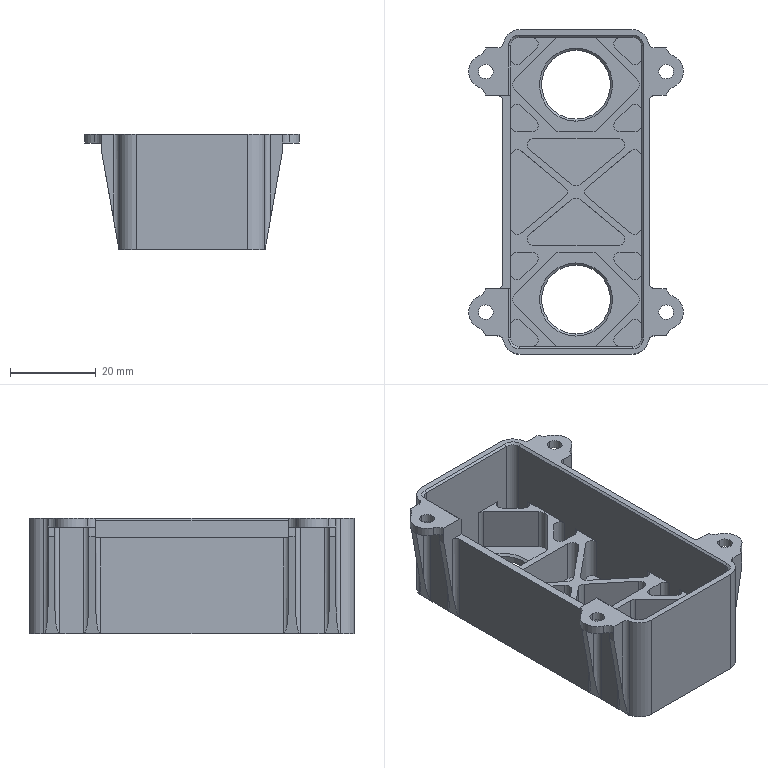NC program | NX | posted with a generic post | part box 50 x 75.58 x 26.8 mm
Lines 6158 to 6975 of 37241:
(ZLEVEL_PROFILE_COPY_1 , TOOL : D6)
N12284 T12 M6
N12286 G54
N12288 G17 G0 G90 X-31.649 Y21.375 S9500 M3
N12290 G43 Z30. H12
N12292 Z-0.992
N12294 G94 G1 X-31.331 Y20.514 F1000.
N12296 G3 X-30.87 Y20.131 R0.6
N12298 G2 X-30.375 Y20. R2.877 F1500.
N12300 G1 X-29.859
N12302 G3 X-29.34 Y20.3 R0.6
N12304 G1 X-28.82 Y21.2
N12306 G0 X-31.525 Y21.463 Z-1.488
N12308 G1 X-31.265 Y20.595 F1000.
N12310 G3 X-30.829 Y20.184 R0.6
N12312 G2 X-30.292 Y20. R2.948 F1500.
N12314 G1 X-29.702
N12316 G3 X-29.183 Y20.3 R0.6
N12318 G1 X-28.663 Y21.2
N12320 G0 X-31.389 Y21.544 Z-1.984
N12322 G1 X-31.177 Y20.662 F1000.
N12324 G3 X-30.764 Y20.227 R0.6
N12326 G2 X-30.208 Y20. R2.99 F1500.
N12328 G1 X-29.571
N12330 G3 X-29.051 Y20.3 R0.6
N12332 G1 X-28.531 Y21.2
N12334 G0 X-31.281 Y21.617 Z-2.48
N12336 G1 X-31.109 Y20.727 F1000.
N12338 G3 X-30.716 Y20.273 R0.6
N12340 G2 X-30.137 Y20. R2.98 F1500.
N12342 G1 X-29.444
N12344 G3 X-28.925 Y20.3 R0.6
N12346 G1 X-28.405 Y21.2
N12348 G0 X-31.183 Y21.686 Z-2.976
N12350 G1 X-31.049 Y20.79 F1000.
N12352 G3 X-30.675 Y20.321 R0.6
N12354 G2 X-30.075 Y20. R2.942 F1500.
N12356 G1 X-29.328
N12358 G3 X-28.809 Y20.3 R0.6
N12360 G1 X-28.289 Y21.2
N12362 G0 X-31.078 Y21.747 Z-3.472
N12364 G1 X-30.977 Y20.846 F1000.
N12366 G3 X-30.622 Y20.363 R0.6
N12368 G2 X-30.007 Y20. R2.977 F1500.
N12370 G1 X-29.216
N12372 G3 X-28.696 Y20.3 R0.6
N12374 G1 X-28.176 Y21.2
N12376 G0 X-30.98 Y21.806 Z-3.968
N12378 G1 X-30.912 Y20.902 F1000.
N12380 G3 X-30.574 Y20.406 R0.6
N12382 G2 X-29.946 Y20. R2.97 F1500.
N12384 G1 X-29.11
N12386 G3 X-28.59 Y20.3 R0.6
N12388 G1 X-28.07 Y21.2
N12390 G0 Z30.
N12392 X-27.167
N12394 Z-0.992
N12396 G1 X-26.647 Y20.3 F1000.
N12398 G3 X-26.128 Y20. R0.6
N12400 G1 X-25.625 F1500.
N12402 G2 X-25.14 Y20.129 R3.02
N12404 G3 X-24.681 Y20.515 R0.6
N12406 G1 X-24.37 Y21.375
N12408 G0 X-27.338 Y21.2 Z-1.488
N12410 G1 X-26.818 Y20.3 F1000.
N12412 G3 X-26.299 Y20. R0.6
N12414 G1 X-25.709 F1500.
N12416 G2 X-25.17 Y20.184 R2.919
N12418 G3 X-24.734 Y20.596 R0.6
N12420 G1 X-24.474 Y21.462
N12422 G0 X-27.469 Y21.2 Z-1.984
N12424 G1 X-26.949 Y20.3 F1000.
N12426 G3 X-26.43 Y20. R0.6
N12428 G1 X-25.788 F1500.
N12430 G2 X-25.23 Y20.229 R2.964
N12432 G3 X-24.816 Y20.664 R0.6
N12434 G1 X-24.604 Y21.544
N12436 G0 X-27.595 Y21.2 Z-2.48
N12438 G1 X-27.075 Y20.3 F1000.
N12440 G3 X-26.556 Y20. R0.6
N12442 G1 X-25.86 F1500.
N12444 G2 X-25.279 Y20.275 R2.952
N12446 G3 X-24.886 Y20.728 R0.6
N12448 G1 X-24.715 Y21.618
N12450 G0 X-27.712 Y21.2 Z-2.976
N12452 G1 X-27.193 Y20.3 F1000.
N12454 G3 X-26.673 Y20. R0.6
N12456 G1 X-25.926 F1500.
N12458 G2 X-25.323 Y20.321 R2.959
N12460 G3 X-24.949 Y20.79 R0.6
N12462 G1 X-24.814 Y21.686
N12464 G0 X-27.823 Y21.2 Z-3.472
N12466 G1 X-27.304 Y20.3 F1000.
N12468 G3 X-26.784 Y20. R0.6
N12470 G1 X-25.994 F1500.
N12472 G2 X-25.38 Y20.362 R2.976
N12474 G3 X-25.024 Y20.845 R0.6
N12476 G1 X-24.924 Y21.746
N12478 G0 X-27.929 Y21.2 Z-3.968
N12480 G1 X-27.41 Y20.3 F1000.
N12482 G3 X-26.89 Y20. R0.6
N12484 G1 X-26.054 F1500.
N12486 G2 X-25.427 Y20.406 R2.97
N12488 G3 X-25.089 Y20.902 R0.6
N12490 G1 X-25.021 Y21.805
N12492 G0 X-28.034 Y21.2 Z-4.464
N12494 G1 X-27.514 Y20.3 F1000.
N12496 G3 X-26.995 Y20. R0.6
N12498 G1 X-26.115 F1500.
N12500 G2 X-25.474 Y20.45 R2.985
N12502 G3 X-25.152 Y20.956 R0.6
N12504 G1 X-25.112 Y21.862
N12506 G0 Z30.
N12508 X-30.888
N12510 Z-4.464
N12512 G1 X-30.848 Y20.956 F1000.
N12514 G3 X-30.526 Y20.45 R0.6
N12516 G2 X-29.885 Y20. R2.985 F1500.
N12518 G1 X-29.005
N12520 G3 X-28.486 Y20.3 R0.6
N12522 G1 X-27.966 Y21.2
N12524 G0 X-30.79 Y21.915 Z-4.96
N12526 G1 X-30.779 Y21.008 F1000.
N12528 G3 X-30.473 Y20.492 R0.6
N12530 G2 X-29.824 Y20. R2.991 F1500.
N12532 G1 X-28.904
N12534 G3 X-28.384 Y20.3 R0.6
N12536 G1 X-27.865 Y21.2
N12538 G0 Z30.
N12540 X-28.135
N12542 Z-4.96
N12544 G1 X-27.615 Y20.3 F1000.
N12546 G3 X-27.096 Y20. R0.6
N12548 G1 X-26.176 F1500.
N12550 G2 X-25.529 Y20.491 R2.984
N12552 G3 X-25.223 Y21.007 R0.6
N12554 G1 X-25.213 Y21.914
N12556 G0 X-28.235 Y21.2 Z-5.456
N12558 G1 X-27.716 Y20.3 F1000.
N12560 G3 X-27.196 Y20. R0.6
N12562 G1 X-26.236 F1500.
N12564 G2 X-25.587 Y20.533 R2.969
N12566 G3 X-25.298 Y21.058 R0.6
N12568 G1 X-25.317 Y21.964
N12570 G0 Z30.
N12572 X-30.691 Y21.965
N12574 Z-5.456
N12576 G1 X-30.708 Y21.058 F1000.
N12578 G3 X-30.417 Y20.533 R0.6
N12580 G2 X-29.764 Y20. R2.988 F1500.
N12582 G1 X-28.804
N12584 G3 X-28.285 Y20.3 R0.6
N12586 G1 X-27.765 Y21.2
N12588 G0 X-30.593 Y22.014 Z-5.952
N12590 G1 X-30.636 Y21.108 F1000.
N12592 G3 X-30.362 Y20.575 R0.6
N12594 G2 X-29.703 Y20. R2.988 F1500.
N12596 G1 X-28.705
N12598 G3 X-28.185 Y20.3 R0.6
N12600 G1 X-27.666 Y21.2
N12602 G0 Z30.
N12604 X-28.334
N12606 Z-5.952
N12608 G1 X-27.815 Y20.3 F1000.
N12610 G3 X-27.295 Y20. R0.6
N12612 G1 X-26.297 F1500.
N12614 G2 X-25.646 Y20.573 R2.962
N12616 G3 X-25.373 Y21.108 R0.6
N12618 G1 X-25.419 Y22.013
N12620 G0 X-28.433 Y21.2 Z-6.448
N12622 G1 X-27.913 Y20.3 F1000.
N12624 G3 X-27.394 Y20. R0.6
N12626 G1 X-26.358 F1500.
N12628 G2 X-25.7 Y20.615 R2.983
N12630 G3 X-25.441 Y21.156 R0.6
N12632 G1 X-25.51 Y22.061
N12634 G0 Z30.
N12636 X-30.497 Y22.062
N12638 Z-6.448
N12640 G1 X-30.564 Y21.157 F1000.
N12642 G3 X-30.304 Y20.617 R0.6
N12644 G2 X-29.642 Y20. R2.997 F1500.
N12646 G1 X-28.606
N12648 G3 X-28.086 Y20.3 R0.6
N12650 G1 X-27.567 Y21.2
N12652 G0 X-30.401 Y22.108 Z-6.944
N12654 G1 X-30.492 Y21.206 F1000.
N12656 G3 X-30.246 Y20.659 R0.6
N12658 G2 X-29.58 Y20. R3.004 F1500.
N12660 G1 X-28.507
N12662 G3 X-27.988 Y20.3 R0.6
N12664 G1 X-27.468 Y21.2
N12666 G0 Z30.
N12668 X-28.532
N12670 Z-6.944
N12672 G1 X-28.012 Y20.3 F1000.
N12674 G3 X-27.493 Y20. R0.6
N12676 G1 X-26.42 F1500.
N12678 G2 X-25.76 Y20.657 R2.99
N12680 G3 X-25.514 Y21.204 R0.6
N12682 G1 X-25.608 Y22.107
N12684 G0 X-28.629 Y21.2 Z-7.44
N12686 G1 X-28.109 Y20.3 F1000.
N12688 G3 X-27.59 Y20. R0.6
N12690 G1 X-26.479 F1500.
N12692 G2 X-25.817 Y20.699 R2.993
N12694 G3 X-25.586 Y21.253 R0.6
N12696 G1 X-25.701 Y22.153
N12698 G0 Z30.
N12700 X-30.307 Y22.155
N12702 Z-7.44
N12704 G1 X-30.42 Y21.255 F1000.
N12706 G3 X-30.188 Y20.702 R0.6
N12708 G2 X-29.521 Y20. R2.998 F1500.
N12710 G1 X-28.41
N12712 G3 X-27.89 Y20.3 R0.6
N12714 G1 X-27.371 Y21.2
N12716 G0 X-30.204 Y22.195 Z-7.936
N12718 G1 X-30.342 Y21.299 F1000.
N12720 G3 X-30.124 Y20.74 R0.6
N12722 G2 X-29.465 Y20. R2.996 F1500.
N12724 G1 X-28.319
N12726 G3 X-27.799 Y20.3 R0.6
N12728 G1 X-27.279 Y21.2
N12730 G0 Z30.
N12732 X-28.722
N12734 Z-7.936
N12736 G1 X-28.202 Y20.3 F1000.
N12738 G3 X-27.682 Y20. R0.6
N12740 G1 X-26.535 F1500.
N12742 G2 X-25.874 Y20.741 R2.994
N12744 G3 X-25.657 Y21.3 R0.6
N12746 G1 X-25.794 Y22.197
N12748 G0 X-28.839 Y21.251 Z-8.432
N12750 G1 X-28.29 Y20.3 F1000.
N12752 G3 X-27.771 Y20. R0.6
N12754 G1 X-26.588 F1500.
N12756 G2 X-25.932 Y20.781 R2.996
N12758 G3 X-25.728 Y21.345 R0.6
N12760 G1 X-25.888 Y22.238
N12762 G0 Z30.
N12764 X-30.115 Y22.24
N12766 Z-8.432
N12768 G1 X-30.274 Y21.347 F1000.
N12770 G3 X-30.07 Y20.782 R0.6
N12772 G2 X-29.412 Y20. R2.996 F1500.
N12774 G1 X-28.229
N12776 G3 X-27.709 Y20.3 R0.6
N12778 G1 X-27.159 Y21.253
N12780 G0 X-30.015 Y22.275 Z-8.928
N12782 G1 X-30.198 Y21.386 F1000.
N12784 G3 X-30.008 Y20.817 R0.6
N12786 G2 X-29.36 Y20. R3.005 F1500.
N12788 G1 X-28.145
N12790 G3 X-27.626 Y20.3 R0.6
N12792 G1 X-26.831 Y21.676
N12794 G0 Z30.
N12796 X-29.169
N12798 Z-8.928
N12800 G1 X-28.374 Y20.3 F1000.
N12802 G3 X-27.855 Y20. R0.6
N12804 G1 X-26.64 F1500.
N12806 G2 X-25.992 Y20.817 R3.005
N12808 G3 X-25.802 Y21.386 R0.6
N12810 G1 X-25.985 Y22.275
N12812 G0 X-29.426 Y21.98 Z-9.424
N12814 G1 X-28.456 Y20.3 F1000.
N12816 G3 X-27.936 Y20. R0.6
N12818 G1 X-26.684 F1500.
N12820 G2 X-26.04 Y20.861 R2.998
N12822 G3 X-25.863 Y21.434 R0.6
N12824 G1 X-26.065 Y22.319
N12826 G0 Z30.
N12828 X-29.935
N12830 Z-9.424
N12832 G1 X-30.137 Y21.434 F1000.
N12834 G3 X-29.96 Y20.861 R0.6
N12836 G2 X-29.316 Y20. R2.998 F1500.
N12838 G1 X-28.064
N12840 G3 X-27.544 Y20.3 R0.6
N12842 G1 X-26.574 Y21.98
N12844 G0 X-29.848 Y22.355 Z-9.92
N12846 G1 X-30.071 Y21.476 F1000.
N12848 G3 X-29.908 Y20.898 R0.6
N12850 G2 X-29.273 Y20. R3.004 F1500.
N12852 G1 X-26.727
N12854 G2 X-26.092 Y20.898 R3.004
N12856 G3 X-25.929 Y21.475 R0.6
N12858 G1 X-26.152 Y22.355
N12860 G0 X-29.772 Y22.396 Z-10.416
N12862 G1 X-30.014 Y21.521 F1000.
N12864 G3 X-29.863 Y20.941 R0.6
N12866 G2 X-29.236 Y20. R3. F1500.
N12868 G1 X-26.765
N12870 G2 X-26.13 Y20.948 R3.003
N12872 G3 X-25.977 Y21.528 R0.6
N12874 G1 X-26.216 Y22.403
N12876 G0 X-29.685 Y22.428 Z-10.912
N12878 G1 X-29.948 Y21.559 F1000.
N12880 G3 X-29.812 Y20.975 R0.6
N12882 G2 X-29.199 Y20. R3.004 F1500.
N12884 G1 X-26.801
N12886 G2 X-26.188 Y20.975 R3.004
N12888 G3 X-26.052 Y21.56 R0.6
N12890 G1 X-26.314 Y22.428
N12892 G0 X-29.634 Y22.481 Z-11.408
N12894 G1 X-29.91 Y21.617 F1000.
N12896 G3 X-29.782 Y21.031 R0.6
N12898 G2 X-29.168 Y20. R3. F1500.
N12900 G1 X-26.832
N12902 G2 X-26.218 Y21.031 R3.
N12904 G3 X-26.09 Y21.617 R0.6
N12906 G1 X-26.366 Y22.481
N12908 G0 X-29.635 Y22.569 Z-11.904
N12910 G1 X-29.91 Y21.704 F1000.
N12912 G3 X-29.782 Y21.118 R0.6
N12914 G2 X-29.139 Y20. R3.002 F1500.
N12916 G1 X-26.861
N12918 G2 X-26.218 Y21.118 R3.003
N12920 G3 X-26.09 Y21.704 R0.6
N12922 G1 X-26.366 Y22.568
N12924 G0 X-29.636 Y22.657 Z-12.4
N12926 G1 X-29.912 Y21.793 F1000.
N12928 G3 X-29.783 Y21.206 R0.6
N12930 G2 X-29.113 Y20. R3.002 F1500.
N12932 G1 X-26.887
N12934 G2 X-26.216 Y21.207 R3.002
N12936 G3 X-26.088 Y21.793 R0.6
N12938 G1 X-26.363 Y22.657
N12940 G0 X-29.635 Y22.744 Z-12.896
N12942 G1 X-29.91 Y21.88 F1000.
N12944 G3 X-29.783 Y21.293 R0.6
N12946 G2 X-29.09 Y20. R3. F1500.
N12948 G1 X-26.91
N12950 G2 X-26.217 Y21.294 R3.
N12952 G3 X-26.089 Y21.88 R0.6
N12954 G1 X-26.365 Y22.744
N12956 G0 X-29.634 Y22.831 Z-13.392
N12958 G1 X-29.91 Y21.967 F1000.
N12960 G3 X-29.782 Y21.38 R0.6
N12962 G2 X-29.069 Y20. R3.001 F1500.
N12964 G1 X-26.931
N12966 G2 X-26.218 Y21.381 R3.001
N12968 G3 X-26.09 Y21.967 R0.6
N12970 G1 X-26.366 Y22.831
N12972 G0 X-29.636 Y22.92 Z-13.888
N12974 G1 X-29.912 Y22.055 F1000.
N12976 G3 X-29.783 Y21.469 R0.6
N12978 G2 X-29.052 Y20. R3. F1500.
N12980 G1 X-26.949
N12982 G2 X-26.217 Y21.468 R3.002
N12984 G3 X-26.089 Y22.055 R0.6
N12986 G1 X-26.364 Y22.919
N12988 G0 X-29.636 Y23.007 Z-14.384
N12990 G1 X-29.912 Y22.142 F1000.
N12992 G3 X-29.783 Y21.556 R0.6
N12994 G2 X-29.036 Y20. R3.004 F1500.
N12996 G1 X-26.964
N12998 G2 X-26.216 Y21.556 R3.003
N13000 G3 X-26.088 Y22.142 R0.6
N13002 G1 X-26.363 Y23.007
N13004 G0 X-29.636 Y23.095 Z-14.88
N13006 G1 X-29.912 Y22.231 F1000.
N13008 G3 X-29.784 Y21.645 R0.6
N13010 G2 X-29.026 Y20. R2.996 F1500.
N13012 G1 X-26.974
N13014 G2 X-26.216 Y21.645 R2.996
N13016 G3 X-26.088 Y22.231 R0.6
N13018 G1 X-26.363 Y23.095
N13020 G0 X-29.638 Y23.184 Z-15.376
N13022 G1 X-29.914 Y22.32 F1000.
N13024 G3 X-29.786 Y21.734 R0.6
N13026 G2 X-29.019 Y20. R2.992 F1500.
N13028 G1 X-26.981
N13030 G2 X-26.214 Y21.734 R2.992
N13032 G3 X-26.086 Y22.32 R0.6
N13034 G1 X-26.362 Y23.184
N13036 G0 X-29.637 Y23.27 Z-15.872
N13038 G1 X-29.912 Y22.406 F1000.
N13040 G3 X-29.784 Y21.819 R0.6
N13042 G2 X-29.008 Y20. R3. F1500.
N13044 G1 X-26.992
N13046 G2 X-26.216 Y21.82 R3.
N13048 G3 X-26.087 Y22.406 R0.6
N13050 G1 X-26.362 Y23.27
N13052 G0 X-29.642 Y23.361 Z-16.368
N13054 G1 X-29.916 Y22.496 F1000.
N13056 G3 X-29.787 Y21.91 R0.6
N13058 G2 X-29.003 Y20. R3.001 F1500.
N13060 G1 X-26.997
N13062 G2 X-26.179 Y21.946 R3.001
N13064 G3 X-26.04 Y22.53 R0.6
N13066 G1 X-26.3 Y23.399
N13068 G0 X-29.635 Y23.444 Z-16.864
N13070 G1 X-29.911 Y22.579 F1000.
N13072 G3 X-29.783 Y21.993 R0.6
N13074 G2 X-29. Y20.033 R3.004 F1500.
N13076 G1 Y20.
N13078 X-27.
N13080 G2 X-26.217 Y21.993 R3.003
N13082 G3 X-26.089 Y22.579 R0.6
N13084 G1 X-26.364 Y23.444
N13086 G0 X-29.647 Y23.537 Z-17.36
N13088 G1 X-29.92 Y22.672 F1000.
N13090 G3 X-29.79 Y22.086 R0.6
N13092 G2 X-29. Y20.061 R3.006 F1500.
N13094 G1 Y20.
N13096 X-27.
N13098 Y20.061
N13100 G2 X-26.209 Y22.087 R3.007
N13102 G3 X-26.079 Y22.673 R0.6
N13104 G1 X-26.351 Y23.538
N13106 G0 X-29.637 Y23.62 Z-17.856
N13108 G1 X-29.912 Y22.755 F1000.
N13110 G3 X-29.784 Y22.169 R0.6
N13112 G2 X-29. Y20.149 R3.003 F1500.
N13114 G1 Y20.
N13116 X-27.
N13118 Y20.149
N13120 G2 X-26.214 Y22.171 R3.004
N13122 G3 X-26.085 Y22.757 R0.6
N13124 G1 X-26.359 Y23.622
N13126 G0 X-29.629 Y23.703 Z-18.352
N13128 G1 X-29.906 Y22.839 F1000.
N13130 G3 X-29.779 Y22.252 R0.6
N13132 G2 X-29. Y20.236 R3. F1500.
N13134 G1 Y20.
N13136 X-27.
N13138 Y20.236
N13140 G2 X-26.221 Y22.253 R3.
N13142 G3 X-26.094 Y22.839 R0.6
N13144 G1 X-26.371 Y23.703
N13146 G0 X-29.629 Y23.79 Z-18.848
N13148 G1 X-29.906 Y22.926 F1000.
N13150 G3 X-29.779 Y22.34 R0.6
N13152 G2 X-29. Y20.323 R3. F1500.
N13154 G1 Y20.
N13156 X-27.
N13158 Y20.323
N13160 G2 X-26.221 Y22.34 R3.
N13162 G3 X-26.094 Y22.926 R0.6
N13164 G1 X-26.371 Y23.79
N13166 G0 X-29.648 Y23.887 Z-19.344
N13168 G1 X-29.92 Y23.022 F1000.
N13170 G3 X-29.79 Y22.436 R0.6
N13172 G2 X-29. Y20.411 R3.006 F1500.
N13174 G1 Y20.
N13176 X-27.
N13178 Y20.411
N13180 G2 X-26.208 Y22.437 R3.007
N13182 G3 X-26.078 Y23.023 R0.6
N13184 G1 X-26.35 Y23.888
N13186 G0 X-29.637 Y23.969 Z-19.84
N13188 G1 X-29.912 Y23.105 F1000.
N13190 G3 X-29.784 Y22.519 R0.6
N13192 G2 X-29. Y20.498 R3.003 F1500.
N13194 G1 Y20.
N13196 X-27.
N13198 Y20.498
N13200 G2 X-26.214 Y22.52 R3.004
N13202 G3 X-26.086 Y23.106 R0.6
N13204 G1 X-26.36 Y23.971
N13206 G0 X-29.637 Y24.057 Z-20.336
N13208 G1 X-29.912 Y23.192 F1000.
N13210 G3 X-29.784 Y22.606 R0.6
N13212 G2 X-29.03 Y21. R3.002 F1500.
N13214 G1 X-29. Y20.586
N13216 Y20.
N13218 X-27.
N13220 Y20.586
N13222 G2 X-26.221 Y22.602 R3.
N13224 G3 X-26.094 Y23.189 R0.6
N13226 G1 X-26.371 Y24.053
N13228 G0 X-29.638 Y24.144 Z-20.832
N13230 G1 X-29.913 Y23.28 F1000.
N13232 G3 X-29.784 Y22.694 R0.6
N13234 G2 X-29. Y20.673 R3.003 F1500.
N13236 G1 Y20.
N13238 X-27.
N13240 Y20.673
N13242 G2 X-26.212 Y22.697 R3.005
N13244 G3 X-26.083 Y23.283 R0.6
N13246 G1 X-26.356 Y24.148
N13248 G0 X-29.653 Y24.24 Z-21.328
N13250 G1 X-29.925 Y23.374 F1000.
N13252 G3 X-29.794 Y22.789 R0.6
N13254 G2 X-29. Y20.761 R3.008 F1500.
N13256 G1 Y20.
N13258 X-27.
N13260 Y20.761
N13262 G2 X-26.208 Y22.787 R3.007
N13264 G3 X-26.078 Y23.373 R0.6
N13266 G1 X-26.35 Y24.238
N13268 G0 X-29.661 Y24.331 Z-21.824
N13270 G1 X-29.93 Y23.465 F1000.
N13272 G3 X-29.798 Y22.879 R0.6
N13274 G2 X-29. Y20.848 R3.011 F1500.
N13276 G1 Y20.
N13278 X-27.
N13280 Y20.848
N13282 G2 X-26.214 Y22.87 R3.004
N13284 G3 X-26.085 Y23.456 R0.6
N13286 G1 X-26.359 Y24.321
N13288 G0 X-29.637 Y24.407 Z-22.32
N13290 G1 X-29.912 Y23.542 F1000.
N13292 G3 X-29.784 Y22.956 R0.6
N13294 G2 X-29. Y20.881 R3.004 F1500.
N13296 G1 Y20.
N13298 X-27.
N13300 Y20.936
N13302 G2 X-26.221 Y22.952 R3.
N13304 G3 X-26.094 Y23.539 R0.6
N13306 G1 X-26.371 Y24.403
N13308 G0 X-29.629 Y24.467 Z-22.816
N13310 G1 X-29.906 Y23.603 F1000.
N13312 G3 X-29.779 Y23.017 R0.6
N13314 G2 X-29. Y21. R3. F1500.
N13316 G1 Y20.
N13318 X-27.
N13320 Y21.
N13322 G2 X-26.221 Y23.017 R3.
N13324 G3 X-26.094 Y23.603 R0.6
N13326 G1 X-26.371 Y24.467
N13328 G0 X-29.629 Z-23.312
N13330 G1 X-29.906 Y23.603 F1000.
N13332 G3 X-29.779 Y23.017 R0.6
N13334 G2 X-29. Y21. R3. F1500.
N13336 G1 Y20.
N13338 X-27.
N13340 Y21.
N13342 G2 X-26.221 Y23.017 R3.
N13344 G3 X-26.094 Y23.603 R0.6
N13346 G1 X-26.371 Y24.467
N13348 G0 X-29.629 Z-23.808
N13350 G1 X-29.906 Y23.603 F1000.
N13352 G3 X-29.779 Y23.017 R0.6
N13354 G2 X-29. Y21. R3. F1500.
N13356 G1 Y20.
N13358 X-27.
N13360 Y21.
N13362 G2 X-26.221 Y23.017 R3.
N13364 G3 X-26.094 Y23.603 R0.6
N13366 G1 X-26.371 Y24.467
N13368 G0 X-29.629 Z-24.304
N13370 G1 X-29.906 Y23.603 F1000.
N13372 G3 X-29.779 Y23.017 R0.6
N13374 G2 X-29. Y21. R3. F1500.
N13376 G1 Y20.
N13378 X-27.
N13380 Y21.
N13382 G2 X-26.221 Y23.017 R3.
N13384 G3 X-26.094 Y23.603 R0.6
N13386 G1 X-26.371 Y24.467
N13388 G0 X-29.629 Z-24.8
N13390 G1 X-29.906 Y23.603 F1000.
N13392 G3 X-29.779 Y23.017 R0.6
N13394 G2 X-29. Y21. R3. F1500.
N13396 G1 Y20.
N13398 X-27.
N13400 Y21.
N13402 G2 X-26.221 Y23.017 R3.
N13404 G3 X-26.094 Y23.603 R0.6
N13406 G1 X-26.371 Y24.467
N13408 G0 Z30.
N13410 X-37.396 Y20.364
N13412 Z-1.984
N13414 G1 X-36.665 Y19.73 F1000.
N13416 G3 X-36.076 Y19.616 R0.6
N13418 G2 X-35.573 Y19.769 R7. F1500.
N13420 G1 X-35.468 Y19.846
N13422 G2 X-35.131 Y20.041 R2.974
N13424 G3 X-34.799 Y20.541 R0.6
N13426 G1 X-34.741 Y21.445
N13428 G0 X-37.507 Y20.309 Z-2.48
N13430 G1 X-36.767 Y19.686 F1000.
N13432 G3 X-36.176 Y19.581 R0.6
N13434 G2 X-35.643 Y19.75 R7. F1500.
N13436 X-35.193 Y20.063 R2.921
N13438 G3 X-34.887 Y20.579 R0.6
N13440 G1 X-34.876 Y21.484
N13442 G0 X-37.606 Y20.258 Z-2.976
N13444 G1 X-36.857 Y19.645 F1000.
N13446 G3 X-36.265 Y19.548 R0.6
N13448 G2 X-35.703 Y19.734 R7. F1500.
N13450 X-35.242 Y20.083 R2.971
N13452 G3 X-34.957 Y20.611 R0.6
N13454 G1 X-34.983 Y21.517
N13456 G0 X-37.708 Y20.204 Z-3.472
N13458 G1 X-36.95 Y19.601 F1000.
N13460 G3 X-36.357 Y19.512 R0.6
N13462 G2 X-35.774 Y19.713 R7. F1500.
N13464 X-35.316 Y20.095 R2.997
N13466 G3 X-35.055 Y20.635 R0.6
N13468 G1 X-35.12 Y21.54
N13470 G0 X-37.804 Y20.151 Z-3.968
N13472 G1 X-37.038 Y19.558 F1000.
N13474 G3 X-36.443 Y19.478 R0.6
N13476 G2 X-35.828 Y19.697 R7. F1500.
N13478 X-35.36 Y20.123 R2.975
N13480 G3 X-35.119 Y20.672 R0.6
N13482 G1 X-35.218 Y21.573
N13484 G0 X-37.896 Y20.098 Z-4.464
N13486 G1 X-37.123 Y19.516 F1000.
N13488 G3 X-36.527 Y19.443 R0.6
N13490 G2 X-35.88 Y19.681 R7. F1500.
N13492 X-35.405 Y20.152 R2.958
N13494 G3 X-35.183 Y20.709 R0.6
N13496 G1 X-35.314 Y21.606
N13498 G0 X-37.98 Y20.049 Z-4.96
N13500 G1 X-37.2 Y19.476 F1000.
N13502 G3 X-36.603 Y19.41 R0.6
N13504 G2 X-35.939 Y19.662 R7. F1500.
N13506 X-35.476 Y20.162 R2.958
N13508 G3 X-35.277 Y20.728 R0.6
N13510 G1 X-35.444 Y21.618
N13512 G0 X-38.07 Y19.995 Z-5.456
N13514 G1 X-37.282 Y19.431 F1000.
N13516 G3 X-36.685 Y19.373 R0.6
N13518 G2 X-36.004 Y19.641 R7. F1500.
N13520 X-35.553 Y20.168 R2.982
N13522 G3 X-35.376 Y20.741 R0.6
N13524 G1 X-35.577 Y21.625
N13526 G0 X-38.157 Y19.94 Z-5.952
N13528 G1 X-37.363 Y19.387 F1000.
N13530 G3 X-36.765 Y19.336 R0.6
N13532 G2 X-36.064 Y19.62 R7. F1500.
N13534 X-35.622 Y20.18 R2.992
N13536 G3 X-35.465 Y20.759 R0.6
N13538 G1 X-35.696 Y21.636
N13540 G0 X-38.25 Y19.881 Z-6.448
N13542 G1 X-37.448 Y19.339 F1000.
N13544 G3 X-36.849 Y19.296 R0.6
N13546 G2 X-36.115 Y19.603 R7. F1500.
N13548 X-35.659 Y20.221 R2.975
N13550 G3 X-35.515 Y20.804 R0.6
N13552 G1 X-35.768 Y21.675
N13554 G0 X-38.333 Y19.827 Z-6.944
N13556 G1 X-37.524 Y19.294 F1000.
N13558 G3 X-36.926 Y19.258 R0.6
N13560 G2 X-36.179 Y19.58 R7. F1500.
N13562 X-35.741 Y20.221 R3.005
N13564 G3 X-35.619 Y20.808 R0.6
N13566 G1 X-35.903 Y21.67
N13568 G0 X-38.407 Y19.777 Z-7.44
N13570 G1 X-37.593 Y19.253 F1000.
N13572 G3 X-36.993 Y19.224 R0.6
N13574 G2 X-36.223 Y19.564 R7. F1500.
N13576 X-35.793 Y20.244 R2.989
N13578 G3 X-35.689 Y20.835 R0.6
N13580 G1 X-35.999 Y21.688
N13582 G0 X-38.477 Y19.729 Z-7.936
N13584 G1 X-37.657 Y19.213 F1000.
N13586 G3 X-37.058 Y19.19 R0.6
N13588 G2 X-36.27 Y19.546 R7. F1500.
N13590 X-35.855 Y20.255 R2.995
N13592 G3 X-35.77 Y20.849 R0.6
N13594 G1 X-36.107 Y21.691
N13596 G0 X-38.539 Y19.685 Z-8.432
N13598 G1 X-37.715 Y19.177 F1000.
N13600 G3 X-37.115 Y19.16 R0.6
N13602 G2 X-36.313 Y19.529 R7. F1500.
N13604 X-35.921 Y20.258 R3.004
N13606 G3 X-35.856 Y20.854 R0.6
N13608 G1 X-36.222 Y21.684
N13610 G0 X-38.599 Y19.642 Z-8.928
N13612 G1 X-37.77 Y19.142 F1000.
N13614 G3 X-37.17 Y19.13 R0.6
N13616 G2 X-36.347 Y19.516 R7. F1500.
N13618 X-35.968 Y20.279 R3.
N13620 G3 X-35.919 Y20.877 R0.6
N13622 G1 X-36.308 Y21.697
N13624 G0 X-38.657 Y19.599 Z-9.424
N13626 G1 X-37.824 Y19.106 F1000.
N13628 G3 X-37.224 Y19.1 R0.6
N13630 G2 X-36.379 Y19.504 R7. F1500.
N13632 X-36.007 Y20.309 R2.999
N13634 G3 X-35.972 Y20.908 R0.6
N13636 G1 X-36.38 Y21.718
N13638 G0 X-38.703 Y19.565 Z-9.92
N13640 G1 X-37.867 Y19.078 F1000.
N13642 G3 X-37.267 Y19.076 R0.6
N13644 G2 X-36.405 Y19.493 R7. F1500.
N13646 X-36.058 Y20.315 R2.999
N13648 G3 X-36.042 Y20.915 R0.6
N13650 G1 X-36.476 Y21.712
N13652 G0 X-38.75 Y19.53 Z-10.416
N13654 G1 X-37.91 Y19.049 F1000.
N13656 G3 X-37.31 Y19.051 R0.6
N13658 G2 X-36.428 Y19.484 R7. F1500.
N13660 X-36.097 Y20.337 R3.
N13662 G3 X-36.097 Y20.937 R0.6
N13664 G1 X-36.55 Y21.723
N13666 G0 X-38.794 Y19.496 Z-10.912
N13668 G1 X-37.951 Y19.02 F1000.
N13670 G3 X-37.351 Y19.026 R0.6
N13672 G2 X-36.448 Y19.476 R7. F1500.
N13674 X-36.131 Y20.365 R3.001
N13676 G3 X-36.144 Y20.965 R0.6
N13678 G1 X-36.615 Y21.74
N13680 G0 X-38.834 Y19.465 Z-11.408
N13682 G1 X-37.988 Y18.995 F1000.
N13684 G3 X-37.388 Y19.005 R0.6
N13686 G2 X-36.462 Y19.47 R7. F1500.
N13688 X-36.159 Y20.398 R2.994
N13690 G3 X-36.186 Y20.997 R0.6
N13692 G1 X-36.674 Y21.761
N13694 G0 X-38.87 Y19.437 Z-11.904
N13696 G1 X-38.021 Y18.972 F1000.
N13698 G3 X-37.421 Y18.985 R0.6
N13700 G2 X-36.474 Y19.465 R7. F1500.
N13702 X-36.19 Y20.424 R2.992
N13704 G3 X-36.23 Y21.022 R0.6
N13706 G1 X-36.736 Y21.775
N13708 G0 X-38.901 Y19.412 Z-12.4
N13710 G1 X-38.05 Y18.951 F1000.
N13712 G3 X-37.451 Y18.967 R0.6
N13714 G2 X-36.486 Y19.46 R7. F1500.
N13716 X-36.219 Y20.445 R3.033
N13718 G3 X-36.272 Y21.043 R0.6
N13720 G1 X-36.795 Y21.786
N13722 G0 X-38.931 Y19.388 Z-12.896
N13724 G1 X-38.078 Y18.93 F1000.
N13726 G3 X-37.479 Y18.949 R0.6
N13728 G2 X-36.493 Y19.457 R7. F1500.
N13730 X-36.25 Y20.467 R3.007
N13732 G3 X-36.317 Y21.063 R0.6
N13734 G1 X-36.857 Y21.793
N13736 G0 X-38.959 Y19.366 Z-13.392
N13738 G1 X-38.104 Y18.912 F1000.
N13740 G3 X-37.504 Y18.933 R0.6
N13742 G2 X-36.499 Y19.455 R7. F1500.
N13744 X-36.274 Y20.495 R3.047
N13746 G3 X-36.355 Y21.09 R0.6
N13748 G1 X-36.911 Y21.808
N13750 G0 X-38.984 Y19.345 Z-13.888
N13752 G1 X-38.127 Y18.895 F1000.
N13754 G3 X-37.527 Y18.919 R0.6
N13756 G2 X-36.499 Y19.455 R7. F1500.
N13758 X-36.303 Y20.516 R2.999
N13760 G3 X-36.398 Y21.109 R0.6
N13762 G1 X-36.971 Y21.812
N13764 G0 X-39.005 Y19.328 Z-14.384
N13766 G1 X-38.146 Y18.881 F1000.
N13768 G3 X-37.547 Y18.906 R0.6
N13770 G2 X-36.5 Y19.454 R7. F1500.
N13772 G1 Y19.536
N13774 G2 X-36.329 Y20.534 R3.
N13776 G3 X-36.44 Y21.123 R0.6
N13778 G1 X-37.03 Y21.812
N13780 G0 X-39.024 Y19.312 Z-14.88
N13782 G1 X-38.164 Y18.867 F1000.
N13784 G3 X-37.565 Y18.895 R0.6
N13786 G2 X-36.5 Y19.454 R7. F1500.
N13788 G1 Y19.624
N13790 G2 X-36.351 Y20.556 R3.
N13792 G3 X-36.475 Y21.143 R0.6
N13794 G1 X-37.081 Y21.819
N13796 G0 X-39.043 Y19.296 Z-15.376
N13798 G1 X-38.182 Y18.854 F1000.
N13800 G3 X-37.583 Y18.883 R0.6
N13802 G2 X-36.5 Y19.454 R7. F1500.
N13804 G1 Y19.711
N13806 G2 X-36.368 Y20.591 R3.
N13808 G3 X-36.502 Y21.176 R0.6
N13810 G1 X-37.12 Y21.84
N13812 G0 X-39.058 Y19.284 Z-15.872
N13814 G1 X-38.196 Y18.843 F1000.
N13816 G3 X-37.597 Y18.874 R0.6
N13818 G2 X-36.5 Y19.454 R7. F1500.
N13820 G1 Y19.799
N13822 G2 X-36.386 Y20.617 R3.
N13824 G3 X-36.533 Y21.199 R0.6
N13826 G1 X-37.165 Y21.849
N13828 G0 X-39.072 Y19.272 Z-16.368
N13830 G1 X-38.209 Y18.834 F1000.
N13832 G3 X-37.61 Y18.866 R0.6
N13834 G2 X-36.5 Y19.454 R7. F1500.
N13836 G1 Y19.886
N13838 G2 X-36.402 Y20.645 R3.
N13840 G3 X-36.561 Y21.224 R0.6
N13842 G1 X-37.206 Y21.862
N13844 G0 X-39.085 Y19.261 Z-16.864
N13846 G1 X-38.221 Y18.824 F1000.
N13848 G3 X-37.622 Y18.858 R0.6
N13850 G2 X-36.5 Y19.454 R7. F1500.
N13852 G1 Y19.974
N13854 G2 X-36.416 Y20.679 R3.
N13856 G3 X-36.585 Y21.255 R0.6
N13858 G1 X-37.242 Y21.881
N13860 G0 X-39.094 Y19.254 Z-17.36
N13862 G1 X-38.229 Y18.818 F1000.
N13864 G3 X-37.63 Y18.853 R0.6
N13866 G2 X-36.5 Y19.454 R7. F1500.
N13868 G1 Y20.061
N13870 G2 X-36.431 Y20.699 R3.
N13872 G3 X-36.614 Y21.271 R0.6
N13874 G1 X-37.285 Y21.881
N13876 G0 X-39.105 Y19.244 Z-17.856
N13878 G1 X-38.24 Y18.81 F1000.
N13880 G3 X-37.641 Y18.846 R0.6
N13882 G2 X-36.5 Y19.454 R7. F1500.
N13884 G1 Y20.149
N13886 G2 X-36.443 Y20.73 R3.
N13888 G3 X-36.637 Y21.298 R0.6
N13890 G1 X-37.319 Y21.896
N13892 G0 X-39.109 Y19.241 Z-18.352
N13894 G1 X-38.243 Y18.807 F1000.
N13896 G3 X-37.645 Y18.843 R0.6
N13898 G2 X-36.5 Y19.454 R7. F1500.
N13900 G1 Y20.236
N13902 G2 X-36.455 Y20.756 R3.
N13904 G3 X-36.66 Y21.32 R0.6
N13906 G1 X-37.355 Y21.903
N13908 G0 X-39.119 Y19.233 Z-18.848
N13910 G1 X-38.252 Y18.801 F1000.
N13912 G3 X-37.653 Y18.837 R0.6